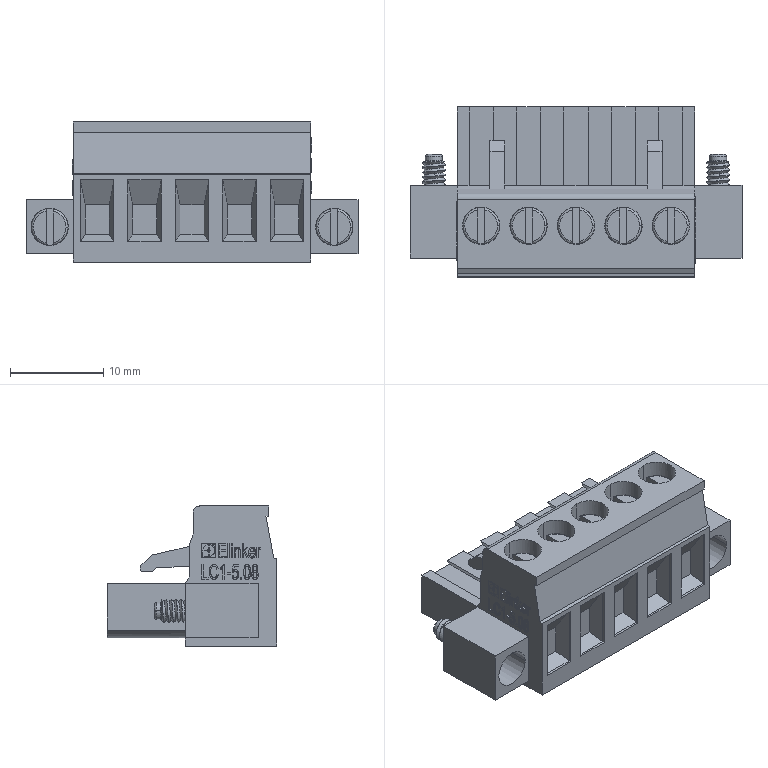Part | NX | features BREP 10 | 10 solids | 2791 faces | box 35.56 x 18.2 x 15 mm | volume 4567 mm3 | plane 2454 | spline 134 | cylinder 125 | torus 64 | cone 14 | commonest cylinder face diameters 2.5 x22 3.9 x14 4 x14 3 x10 0.443 x6 5.34 x5